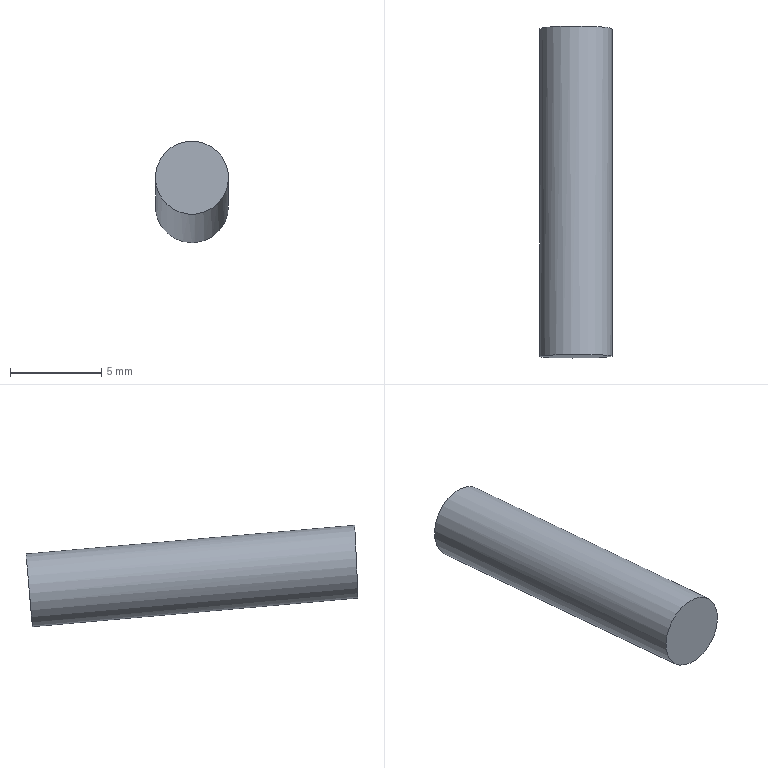Part | NX | features solid 2 | 1 solid | 3 faces | box 4 x 18.167 x 5.558 mm | volume 225.816 mm3 | plane 2 | cylinder 1 | commonest cylinder face diameters 4 x1
STEP:
#1=CARTESIAN_POINT('',(-120.452,-28.179,-29.547));
#2=VERTEX_POINT('',#1);
#3=CARTESIAN_POINT('',(-120.452,-28.005,-27.555));
#4=DIRECTION('',(0.,-0.9962,0.08716));
#5=DIRECTION('',(0.,-0.08716,-0.9962));
#6=AXIS2_PLACEMENT_3D('',#3,#4,#5);
#7=CIRCLE('',#6,2.);
#8=EDGE_CURVE('',#2,#2,#7,.T.);
#9=ORIENTED_EDGE('',*,*,#8,.F.);
#10=EDGE_LOOP('',(#9));
#11=FACE_BOUND('',#10,.T.);
#12=CARTESIAN_POINT('',(-120.452,-28.005,-27.555));
#13=DIRECTION('',(0.,0.9962,-0.08716));
#14=DIRECTION('',(0.,0.08716,0.9962));
#15=AXIS2_PLACEMENT_3D('',#12,#13,#14);
#16=PLANE('',#15);
#17=ADVANCED_FACE('',(#11),#16,.T.);
#18=CARTESIAN_POINT('',(-120.266,-45.996,-27.98));
#19=VERTEX_POINT('',#18);
#20=CARTESIAN_POINT('',(-120.452,-45.906,-25.989));
#21=DIRECTION('',(0.00391,-0.999,0.04549));
#22=DIRECTION('',(0.09317,-0.04493,-0.9946));
#23=AXIS2_PLACEMENT_3D('',#20,#21,#22);
#24=ELLIPSE('',#23,2.002,2.);
#25=EDGE_CURVE('',#19,#19,#24,.F.);
#26=ORIENTED_EDGE('',*,*,#25,.F.);
#27=EDGE_LOOP('',(#26));
#28=FACE_BOUND('',#27,.T.);
#29=CARTESIAN_POINT('',(-78.701,-48.763,-92.296));
#30=DIRECTION('',(0.00391,-0.999,0.04549));
#31=DIRECTION('',(-0.05224,0.04523,0.9976));
#32=AXIS2_PLACEMENT_3D('',#29,#30,#31);
#33=PLANE('',#32);
#34=ADVANCED_FACE('',(#28),#33,.T.);
#35=ORIENTED_EDGE('',*,*,#8,.T.);
#36=EDGE_LOOP('',(#35));
#37=FACE_BOUND('',#36,.T.);
#38=ORIENTED_EDGE('',*,*,#25,.T.);
#39=EDGE_LOOP('',(#38));
#40=FACE_BOUND('',#39,.T.);
#41=CARTESIAN_POINT('',(-120.452,-47.929,-25.812));
#42=DIRECTION('',(0.,0.9962,-0.08716));
#43=DIRECTION('',(0.,0.08716,0.9962));
#44=AXIS2_PLACEMENT_3D('',#41,#42,#43);
#45=CYLINDRICAL_SURFACE('',#44,2.);
#46=ADVANCED_FACE('',(#37,#40),#45,.T.);
#47=CLOSED_SHELL('',(#17,#34,#46));
#48=MANIFOLD_SOLID_BREP('',#47);
#49=(LENGTH_UNIT()NAMED_UNIT(*)SI_UNIT(.MILLI.,.METRE.));
#50=UNCERTAINTY_MEASURE_WITH_UNIT(LENGTH_MEASURE(0.00001),#49,'','');
#51=(NAMED_UNIT(*)PLANE_ANGLE_UNIT()SI_UNIT($,.RADIAN.));
#52=(NAMED_UNIT(*)SI_UNIT($,.STERADIAN.)SOLID_ANGLE_UNIT());
#53=(GEOMETRIC_REPRESENTATION_CONTEXT(3)GLOBAL_UNCERTAINTY_ASSIGNED_CONTEXT((#50))GLOBAL_UNIT_ASSIGNED_CONTEXT((#49,#51,#52))REPRESENTATION_CONTEXT('',''));
#54=ADVANCED_BREP_SHAPE_REPRESENTATION('',(#48),#53);